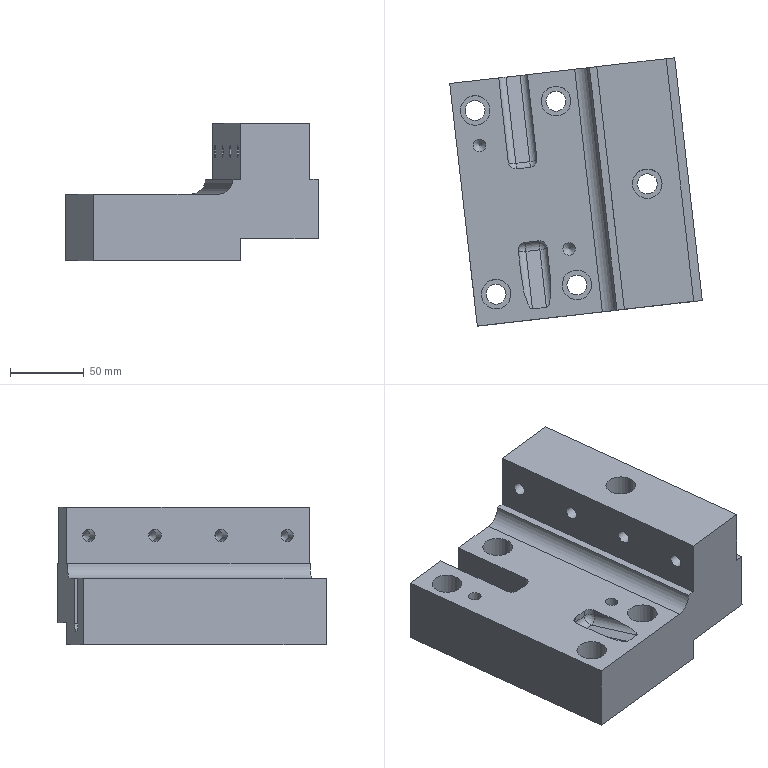Part | NX | features XQ 2 | 1 solid | 67 faces | box 170.695 x 181.259 x 93 mm | volume 1290279 mm3 | cylinder 29 | plane 26 | cone 8 | sphere 4 | commonest cylinder face diameters 10 x10 8.5 x8 20 x6 13.5 x5